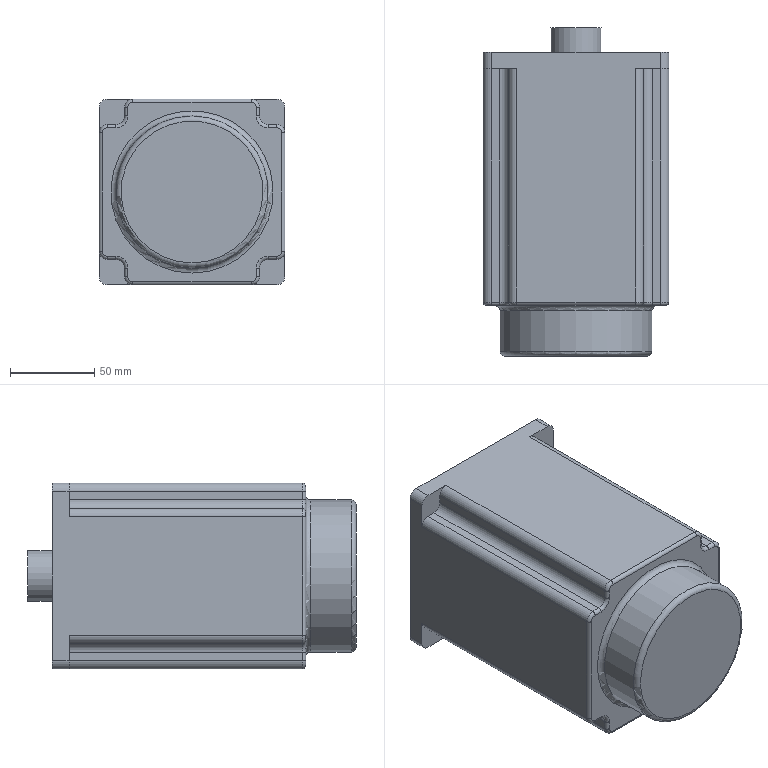Part | STEP file | Tube feed_id130_x_t | 1 solid | 64 faces | box 110 x 194.5 x 110 mm | volume 1886545 mm3 | cylinder 30 | plane 20 | torus 14 | commonest cylinder face diameters 10 x16 4 x12 30 x1 90 x1